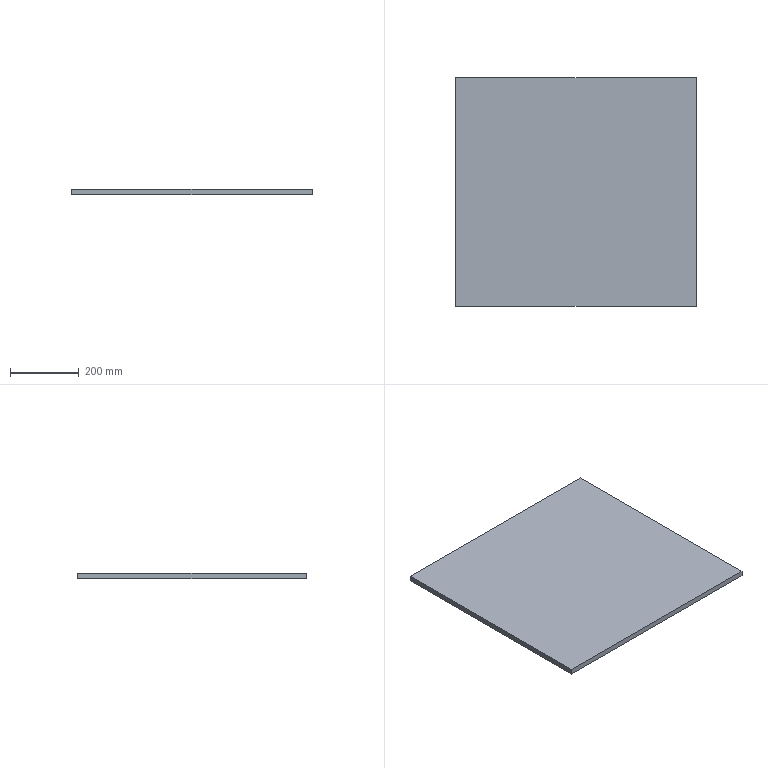Part | STEP file | Small table plate | 1 solid | 6 faces | box 700 x 665 x 16 mm | volume 7448000 mm3 | plane 6
STEP:
#1=CARTESIAN_POINT('',(0.,0.,0.));
#2=DIRECTION('',(0.,0.,1.));
#3=DIRECTION('',(1.,0.,0.));
#4=AXIS2_PLACEMENT_3D('',#1,#2,#3);
#5=CARTESIAN_POINT('',(-350.,332.5,16.));
#6=VERTEX_POINT('',#5);
#7=CARTESIAN_POINT('',(-350.,-332.5,16.));
#8=VERTEX_POINT('',#7);
#9=CARTESIAN_POINT('',(-350.,0.,16.));
#10=DIRECTION('',(0.,-1.,0.));
#11=VECTOR('',#10,1.);
#12=LINE('',#9,#11);
#13=CARTESIAN_POINT('',(0.,0.,16.));
#14=DIRECTION('',(0.,0.,1.));
#15=DIRECTION('',(1.,0.,0.));
#16=AXIS2_PLACEMENT_3D('',#13,#14,#15);
#17=PLANE('',#16);
#18=CARTESIAN_POINT('',(-350.,0.));
#19=DIRECTION('',(0.,-1.));
#20=VECTOR('',#19,1.);
#21=LINE('',#18,#20);
#22=(GEOMETRIC_REPRESENTATION_CONTEXT(2)PARAMETRIC_REPRESENTATION_CONTEXT()REPRESENTATION_CONTEXT('',''));
#23=DEFINITIONAL_REPRESENTATION('',(#21),#22);
#24=PCURVE('',#17,#23);
#25=CARTESIAN_POINT('',(-350.,332.5,16.));
#26=DIRECTION('',(1.,0.,0.));
#27=DIRECTION('',(0.,1.,0.));
#28=AXIS2_PLACEMENT_3D('',#25,#26,#27);
#29=PLANE('',#28);
#30=CARTESIAN_POINT('',(-332.5,0.));
#31=DIRECTION('',(-1.,0.));
#32=VECTOR('',#31,1.);
#33=LINE('',#30,#32);
#34=(GEOMETRIC_REPRESENTATION_CONTEXT(2)PARAMETRIC_REPRESENTATION_CONTEXT()REPRESENTATION_CONTEXT('',''));
#35=DEFINITIONAL_REPRESENTATION('',(#33),#34);
#36=PCURVE('',#29,#35);
#37=SURFACE_CURVE('',#12,(#24,#36),.PCURVE_S1.);
#38=EDGE_CURVE('',#6,#8,#37,.T.);
#39=ORIENTED_EDGE('',*,*,#38,.T.);
#40=CARTESIAN_POINT('',(350.,-332.5,16.));
#41=VERTEX_POINT('',#40);
#42=CARTESIAN_POINT('',(0.,-332.5,16.));
#43=DIRECTION('',(1.,0.,0.));
#44=VECTOR('',#43,1.);
#45=LINE('',#42,#44);
#46=CARTESIAN_POINT('',(0.,-332.5));
#47=DIRECTION('',(1.,0.));
#48=VECTOR('',#47,1.);
#49=LINE('',#46,#48);
#50=(GEOMETRIC_REPRESENTATION_CONTEXT(2)PARAMETRIC_REPRESENTATION_CONTEXT()REPRESENTATION_CONTEXT('',''));
#51=DEFINITIONAL_REPRESENTATION('',(#49),#50);
#52=PCURVE('',#17,#51);
#53=CARTESIAN_POINT('',(-350.,-332.5,16.));
#54=DIRECTION('',(0.,1.,0.));
#55=DIRECTION('',(0.,0.,1.));
#56=AXIS2_PLACEMENT_3D('',#53,#54,#55);
#57=PLANE('',#56);
#58=CARTESIAN_POINT('',(0.,350.));
#59=DIRECTION('',(0.,1.));
#60=VECTOR('',#59,1.);
#61=LINE('',#58,#60);
#62=(GEOMETRIC_REPRESENTATION_CONTEXT(2)PARAMETRIC_REPRESENTATION_CONTEXT()REPRESENTATION_CONTEXT('',''));
#63=DEFINITIONAL_REPRESENTATION('',(#61),#62);
#64=PCURVE('',#57,#63);
#65=SURFACE_CURVE('',#45,(#52,#64),.PCURVE_S1.);
#66=EDGE_CURVE('',#8,#41,#65,.T.);
#67=ORIENTED_EDGE('',*,*,#66,.T.);
#68=CARTESIAN_POINT('',(350.,332.5,16.));
#69=VERTEX_POINT('',#68);
#70=CARTESIAN_POINT('',(350.,0.,16.));
#71=DIRECTION('',(0.,1.,0.));
#72=VECTOR('',#71,1.);
#73=LINE('',#70,#72);
#74=CARTESIAN_POINT('',(350.,0.));
#75=DIRECTION('',(0.,1.));
#76=VECTOR('',#75,1.);
#77=LINE('',#74,#76);
#78=(GEOMETRIC_REPRESENTATION_CONTEXT(2)PARAMETRIC_REPRESENTATION_CONTEXT()REPRESENTATION_CONTEXT('',''));
#79=DEFINITIONAL_REPRESENTATION('',(#77),#78);
#80=PCURVE('',#17,#79);
#81=CARTESIAN_POINT('',(350.,332.5,16.));
#82=DIRECTION('',(-1.,0.,0.));
#83=DIRECTION('',(0.,-1.,0.));
#84=AXIS2_PLACEMENT_3D('',#81,#82,#83);
#85=PLANE('',#84);
#86=CARTESIAN_POINT('',(332.5,0.));
#87=DIRECTION('',(-1.,0.));
#88=VECTOR('',#87,1.);
#89=LINE('',#86,#88);
#90=(GEOMETRIC_REPRESENTATION_CONTEXT(2)PARAMETRIC_REPRESENTATION_CONTEXT()REPRESENTATION_CONTEXT('',''));
#91=DEFINITIONAL_REPRESENTATION('',(#89),#90);
#92=PCURVE('',#85,#91);
#93=SURFACE_CURVE('',#73,(#80,#92),.PCURVE_S1.);
#94=EDGE_CURVE('',#41,#69,#93,.T.);
#95=ORIENTED_EDGE('',*,*,#94,.T.);
#96=CARTESIAN_POINT('',(0.,332.5,16.));
#97=DIRECTION('',(-1.,0.,0.));
#98=VECTOR('',#97,1.);
#99=LINE('',#96,#98);
#100=CARTESIAN_POINT('',(0.,332.5));
#101=DIRECTION('',(-1.,0.));
#102=VECTOR('',#101,1.);
#103=LINE('',#100,#102);
#104=(GEOMETRIC_REPRESENTATION_CONTEXT(2)PARAMETRIC_REPRESENTATION_CONTEXT()REPRESENTATION_CONTEXT('',''));
#105=DEFINITIONAL_REPRESENTATION('',(#103),#104);
#106=PCURVE('',#17,#105);
#107=CARTESIAN_POINT('',(-350.,332.5,16.));
#108=DIRECTION('',(0.,-1.,0.));
#109=DIRECTION('',(0.,0.,-1.));
#110=AXIS2_PLACEMENT_3D('',#107,#108,#109);
#111=PLANE('',#110);
#112=CARTESIAN_POINT('',(0.,350.));
#113=DIRECTION('',(0.,-1.));
#114=VECTOR('',#113,1.);
#115=LINE('',#112,#114);
#116=(GEOMETRIC_REPRESENTATION_CONTEXT(2)PARAMETRIC_REPRESENTATION_CONTEXT()REPRESENTATION_CONTEXT('',''));
#117=DEFINITIONAL_REPRESENTATION('',(#115),#116);
#118=PCURVE('',#111,#117);
#119=SURFACE_CURVE('',#99,(#106,#118),.PCURVE_S1.);
#120=EDGE_CURVE('',#69,#6,#119,.T.);
#121=ORIENTED_EDGE('',*,*,#120,.T.);
#122=EDGE_LOOP('',(#39,#67,#95,#121));
#123=FACE_BOUND('',#122,.T.);
#124=ADVANCED_FACE('',(#123),#17,.T.);
#125=CARTESIAN_POINT('',(350.,-332.5,0.));
#126=VERTEX_POINT('',#125);
#127=CARTESIAN_POINT('',(350.,-332.5,16.));
#128=DIRECTION('',(0.,0.,-1.));
#129=VECTOR('',#128,1.);
#130=LINE('',#127,#129);
#131=CARTESIAN_POINT('',(0.,700.));
#132=DIRECTION('',(-1.,0.));
#133=VECTOR('',#132,1.);
#134=LINE('',#131,#133);
#135=(GEOMETRIC_REPRESENTATION_CONTEXT(2)PARAMETRIC_REPRESENTATION_CONTEXT()REPRESENTATION_CONTEXT('',''));
#136=DEFINITIONAL_REPRESENTATION('',(#134),#135);
#137=PCURVE('',#57,#136);
#138=CARTESIAN_POINT('',(665.,0.));
#139=DIRECTION('',(0.,-1.));
#140=VECTOR('',#139,1.);
#141=LINE('',#138,#140);
#142=(GEOMETRIC_REPRESENTATION_CONTEXT(2)PARAMETRIC_REPRESENTATION_CONTEXT()REPRESENTATION_CONTEXT('',''));
#143=DEFINITIONAL_REPRESENTATION('',(#141),#142);
#144=PCURVE('',#85,#143);
#145=SURFACE_CURVE('',#130,(#137,#144),.PCURVE_S1.);
#146=EDGE_CURVE('',#41,#126,#145,.T.);
#147=ORIENTED_EDGE('',*,*,#146,.F.);
#148=ORIENTED_EDGE('',*,*,#66,.F.);
#149=CARTESIAN_POINT('',(-350.,-332.5,0.));
#150=VERTEX_POINT('',#149);
#151=CARTESIAN_POINT('',(-350.,-332.5,16.));
#152=DIRECTION('',(0.,0.,1.));
#153=VECTOR('',#152,1.);
#154=LINE('',#151,#153);
#155=CARTESIAN_POINT('',(0.,0.));
#156=DIRECTION('',(1.,0.));
#157=VECTOR('',#156,1.);
#158=LINE('',#155,#157);
#159=(GEOMETRIC_REPRESENTATION_CONTEXT(2)PARAMETRIC_REPRESENTATION_CONTEXT()REPRESENTATION_CONTEXT('',''));
#160=DEFINITIONAL_REPRESENTATION('',(#158),#159);
#161=PCURVE('',#57,#160);
#162=CARTESIAN_POINT('',(-665.,0.));
#163=DIRECTION('',(0.,1.));
#164=VECTOR('',#163,1.);
#165=LINE('',#162,#164);
#166=(GEOMETRIC_REPRESENTATION_CONTEXT(2)PARAMETRIC_REPRESENTATION_CONTEXT()REPRESENTATION_CONTEXT('',''));
#167=DEFINITIONAL_REPRESENTATION('',(#165),#166);
#168=PCURVE('',#29,#167);
#169=SURFACE_CURVE('',#154,(#161,#168),.PCURVE_S1.);
#170=EDGE_CURVE('',#150,#8,#169,.T.);
#171=ORIENTED_EDGE('',*,*,#170,.F.);
#172=CARTESIAN_POINT('',(-350.,-332.5,0.));
#173=DIRECTION('',(-1.,0.,0.));
#174=VECTOR('',#173,1.);
#175=LINE('',#172,#174);
#176=CARTESIAN_POINT('',(-16.,0.));
#177=DIRECTION('',(0.,-1.));
#178=VECTOR('',#177,1.);
#179=LINE('',#176,#178);
#180=(GEOMETRIC_REPRESENTATION_CONTEXT(2)PARAMETRIC_REPRESENTATION_CONTEXT()REPRESENTATION_CONTEXT('',''));
#181=DEFINITIONAL_REPRESENTATION('',(#179),#180);
#182=PCURVE('',#57,#181);
#183=CARTESIAN_POINT('',(0.,0.,0.));
#184=DIRECTION('',(0.,0.,1.));
#185=DIRECTION('',(1.,0.,0.));
#186=AXIS2_PLACEMENT_3D('',#183,#184,#185);
#187=PLANE('',#186);
#188=CARTESIAN_POINT('',(-350.,-332.5));
#189=DIRECTION('',(-1.,0.));
#190=VECTOR('',#189,1.);
#191=LINE('',#188,#190);
#192=(GEOMETRIC_REPRESENTATION_CONTEXT(2)PARAMETRIC_REPRESENTATION_CONTEXT()REPRESENTATION_CONTEXT('',''));
#193=DEFINITIONAL_REPRESENTATION('',(#191),#192);
#194=PCURVE('',#187,#193);
#195=SURFACE_CURVE('',#175,(#182,#194),.PCURVE_S1.);
#196=EDGE_CURVE('',#126,#150,#195,.T.);
#197=ORIENTED_EDGE('',*,*,#196,.F.);
#198=EDGE_LOOP('',(#147,#148,#171,#197));
#199=FACE_BOUND('',#198,.T.);
#200=ADVANCED_FACE('',(#199),#57,.F.);
#201=ORIENTED_EDGE('',*,*,#170,.T.);
#202=ORIENTED_EDGE('',*,*,#38,.F.);
#203=CARTESIAN_POINT('',(-350.,332.5,0.));
#204=VERTEX_POINT('',#203);
#205=CARTESIAN_POINT('',(-350.,332.5,16.));
#206=DIRECTION('',(0.,0.,1.));
#207=VECTOR('',#206,1.);
#208=LINE('',#205,#207);
#209=CARTESIAN_POINT('',(0.,0.));
#210=DIRECTION('',(0.,1.));
#211=VECTOR('',#210,1.);
#212=LINE('',#209,#211);
#213=(GEOMETRIC_REPRESENTATION_CONTEXT(2)PARAMETRIC_REPRESENTATION_CONTEXT()REPRESENTATION_CONTEXT('',''));
#214=DEFINITIONAL_REPRESENTATION('',(#212),#213);
#215=PCURVE('',#29,#214);
#216=CARTESIAN_POINT('',(0.,0.));
#217=DIRECTION('',(-1.,0.));
#218=VECTOR('',#217,1.);
#219=LINE('',#216,#218);
#220=(GEOMETRIC_REPRESENTATION_CONTEXT(2)PARAMETRIC_REPRESENTATION_CONTEXT()REPRESENTATION_CONTEXT('',''));
#221=DEFINITIONAL_REPRESENTATION('',(#219),#220);
#222=PCURVE('',#111,#221);
#223=SURFACE_CURVE('',#208,(#215,#222),.PCURVE_S1.);
#224=EDGE_CURVE('',#204,#6,#223,.T.);
#225=ORIENTED_EDGE('',*,*,#224,.F.);
#226=CARTESIAN_POINT('',(-350.,332.5,0.));
#227=DIRECTION('',(0.,1.,0.));
#228=VECTOR('',#227,1.);
#229=LINE('',#226,#228);
#230=CARTESIAN_POINT('',(0.,-16.));
#231=DIRECTION('',(1.,0.));
#232=VECTOR('',#231,1.);
#233=LINE('',#230,#232);
#234=(GEOMETRIC_REPRESENTATION_CONTEXT(2)PARAMETRIC_REPRESENTATION_CONTEXT()REPRESENTATION_CONTEXT('',''));
#235=DEFINITIONAL_REPRESENTATION('',(#233),#234);
#236=PCURVE('',#29,#235);
#237=CARTESIAN_POINT('',(-350.,332.5));
#238=DIRECTION('',(0.,1.));
#239=VECTOR('',#238,1.);
#240=LINE('',#237,#239);
#241=(GEOMETRIC_REPRESENTATION_CONTEXT(2)PARAMETRIC_REPRESENTATION_CONTEXT()REPRESENTATION_CONTEXT('',''));
#242=DEFINITIONAL_REPRESENTATION('',(#240),#241);
#243=PCURVE('',#187,#242);
#244=SURFACE_CURVE('',#229,(#236,#243),.PCURVE_S1.);
#245=EDGE_CURVE('',#150,#204,#244,.T.);
#246=ORIENTED_EDGE('',*,*,#245,.F.);
#247=EDGE_LOOP('',(#201,#202,#225,#246));
#248=FACE_BOUND('',#247,.T.);
#249=ADVANCED_FACE('',(#248),#29,.F.);
#250=ORIENTED_EDGE('',*,*,#224,.T.);
#251=ORIENTED_EDGE('',*,*,#120,.F.);
#252=CARTESIAN_POINT('',(350.,332.5,0.));
#253=VERTEX_POINT('',#252);
#254=CARTESIAN_POINT('',(350.,332.5,16.));
#255=DIRECTION('',(0.,0.,1.));
#256=VECTOR('',#255,1.);
#257=LINE('',#254,#256);
#258=CARTESIAN_POINT('',(0.,700.));
#259=DIRECTION('',(-1.,0.));
#260=VECTOR('',#259,1.);
#261=LINE('',#258,#260);
#262=(GEOMETRIC_REPRESENTATION_CONTEXT(2)PARAMETRIC_REPRESENTATION_CONTEXT()REPRESENTATION_CONTEXT('',''));
#263=DEFINITIONAL_REPRESENTATION('',(#261),#262);
#264=PCURVE('',#111,#263);
#265=CARTESIAN_POINT('',(0.,0.));
#266=DIRECTION('',(0.,1.));
#267=VECTOR('',#266,1.);
#268=LINE('',#265,#267);
#269=(GEOMETRIC_REPRESENTATION_CONTEXT(2)PARAMETRIC_REPRESENTATION_CONTEXT()REPRESENTATION_CONTEXT('',''));
#270=DEFINITIONAL_REPRESENTATION('',(#268),#269);
#271=PCURVE('',#85,#270);
#272=SURFACE_CURVE('',#257,(#264,#271),.PCURVE_S1.);
#273=EDGE_CURVE('',#253,#69,#272,.T.);
#274=ORIENTED_EDGE('',*,*,#273,.F.);
#275=CARTESIAN_POINT('',(-350.,332.5,0.));
#276=DIRECTION('',(1.,0.,0.));
#277=VECTOR('',#276,1.);
#278=LINE('',#275,#277);
#279=CARTESIAN_POINT('',(16.,0.));
#280=DIRECTION('',(0.,1.));
#281=VECTOR('',#280,1.);
#282=LINE('',#279,#281);
#283=(GEOMETRIC_REPRESENTATION_CONTEXT(2)PARAMETRIC_REPRESENTATION_CONTEXT()REPRESENTATION_CONTEXT('',''));
#284=DEFINITIONAL_REPRESENTATION('',(#282),#283);
#285=PCURVE('',#111,#284);
#286=CARTESIAN_POINT('',(-350.,332.5));
#287=DIRECTION('',(1.,0.));
#288=VECTOR('',#287,1.);
#289=LINE('',#286,#288);
#290=(GEOMETRIC_REPRESENTATION_CONTEXT(2)PARAMETRIC_REPRESENTATION_CONTEXT()REPRESENTATION_CONTEXT('',''));
#291=DEFINITIONAL_REPRESENTATION('',(#289),#290);
#292=PCURVE('',#187,#291);
#293=SURFACE_CURVE('',#278,(#285,#292),.PCURVE_S1.);
#294=EDGE_CURVE('',#204,#253,#293,.T.);
#295=ORIENTED_EDGE('',*,*,#294,.F.);
#296=EDGE_LOOP('',(#250,#251,#274,#295));
#297=FACE_BOUND('',#296,.T.);
#298=ADVANCED_FACE('',(#297),#111,.F.);
#299=ORIENTED_EDGE('',*,*,#273,.T.);
#300=ORIENTED_EDGE('',*,*,#94,.F.);
#301=ORIENTED_EDGE('',*,*,#146,.T.);
#302=CARTESIAN_POINT('',(350.,332.5,0.));
#303=DIRECTION('',(0.,-1.,0.));
#304=VECTOR('',#303,1.);
#305=LINE('',#302,#304);
#306=CARTESIAN_POINT('',(0.,-16.));
#307=DIRECTION('',(1.,0.));
#308=VECTOR('',#307,1.);
#309=LINE('',#306,#308);
#310=(GEOMETRIC_REPRESENTATION_CONTEXT(2)PARAMETRIC_REPRESENTATION_CONTEXT()REPRESENTATION_CONTEXT('',''));
#311=DEFINITIONAL_REPRESENTATION('',(#309),#310);
#312=PCURVE('',#85,#311);
#313=CARTESIAN_POINT('',(350.,332.5));
#314=DIRECTION('',(0.,-1.));
#315=VECTOR('',#314,1.);
#316=LINE('',#313,#315);
#317=(GEOMETRIC_REPRESENTATION_CONTEXT(2)PARAMETRIC_REPRESENTATION_CONTEXT()REPRESENTATION_CONTEXT('',''));
#318=DEFINITIONAL_REPRESENTATION('',(#316),#317);
#319=PCURVE('',#187,#318);
#320=SURFACE_CURVE('',#305,(#312,#319),.PCURVE_S1.);
#321=EDGE_CURVE('',#253,#126,#320,.T.);
#322=ORIENTED_EDGE('',*,*,#321,.F.);
#323=EDGE_LOOP('',(#299,#300,#301,#322));
#324=FACE_BOUND('',#323,.T.);
#325=ADVANCED_FACE('',(#324),#85,.F.);
#326=ORIENTED_EDGE('',*,*,#196,.T.);
#327=ORIENTED_EDGE('',*,*,#245,.T.);
#328=ORIENTED_EDGE('',*,*,#294,.T.);
#329=ORIENTED_EDGE('',*,*,#321,.T.);
#330=EDGE_LOOP('',(#326,#327,#328,#329));
#331=FACE_BOUND('',#330,.T.);
#332=ADVANCED_FACE('',(#331),#187,.F.);
#333=CLOSED_SHELL('',(#124,#200,#249,#298,#325,#332));
#334=MANIFOLD_SOLID_BREP('',#333);
#335=(LENGTH_UNIT()NAMED_UNIT(*)SI_UNIT(.MILLI.,.METRE.));
#336=UNCERTAINTY_MEASURE_WITH_UNIT(LENGTH_MEASURE(0.0000001),#335,'','');
#337=(NAMED_UNIT(*)PLANE_ANGLE_UNIT()SI_UNIT($,.RADIAN.));
#338=(NAMED_UNIT(*)SI_UNIT($,.STERADIAN.)SOLID_ANGLE_UNIT());
#339=(GEOMETRIC_REPRESENTATION_CONTEXT(3)GLOBAL_UNCERTAINTY_ASSIGNED_CONTEXT((#336))GLOBAL_UNIT_ASSIGNED_CONTEXT((#335,#337,#338))REPRESENTATION_CONTEXT('',''));
#340=ADVANCED_BREP_SHAPE_REPRESENTATION('',(#4,#334),#339);